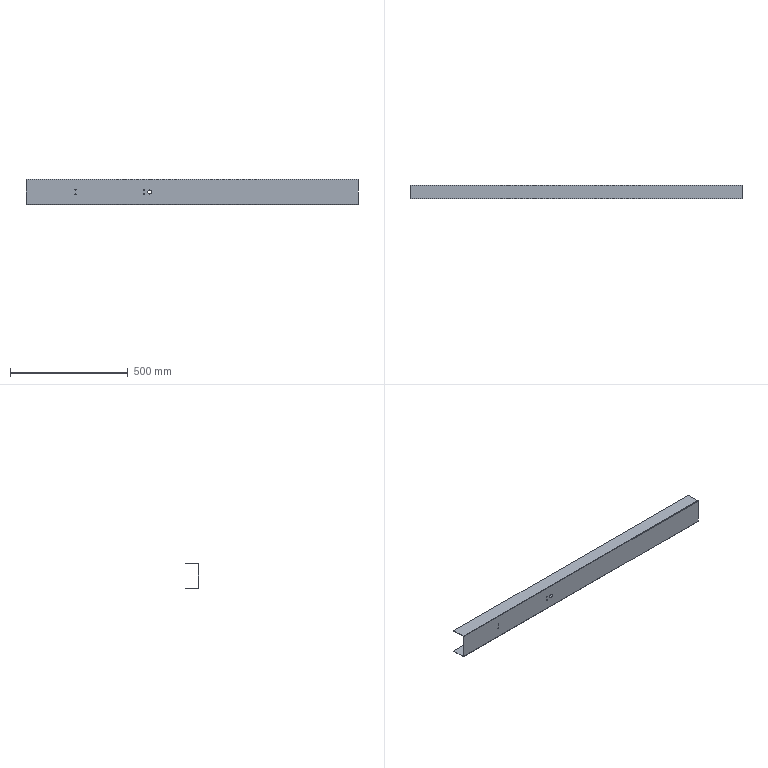Part | STEP file | Trunking Light 5 | 1 solid | 24 faces | box 1408 x 58 x 107 mm | volume 462641 mm3 | cylinder 14 | plane 10 | commonest cylinder face diameters 5 x8 0.2 x2 3.2 x2 17 x2
STEP:
#1=CARTESIAN_POINT('',(525.,-37.727,-23.631));
#2=VERTEX_POINT('',#1);
#3=CARTESIAN_POINT('',(525.,-37.727,-40.631));
#4=VERTEX_POINT('',#3);
#5=CARTESIAN_POINT('',(525.,-37.727,-32.131));
#6=DIRECTION('',(0.,-1.,0.));
#7=DIRECTION('',(0.,0.,-1.));
#8=AXIS2_PLACEMENT_3D('',#5,#6,#7);
#9=CIRCLE('',#8,8.5);
#10=EDGE_CURVE('',#2,#4,#9,.T.);
#11=ORIENTED_EDGE('',*,*,#10,.F.);
#12=CARTESIAN_POINT('',(525.,-39.227,-23.631));
#13=VERTEX_POINT('',#12);
#14=CARTESIAN_POINT('',(525.,-29.227,-23.631));
#15=DIRECTION('',(0.,-1.,0.));
#16=VECTOR('',#15,1000.);
#17=LINE('',#14,#16);
#18=EDGE_CURVE('',#2,#13,#17,.T.);
#19=ORIENTED_EDGE('',*,*,#18,.T.);
#20=CARTESIAN_POINT('',(525.,-39.227,-40.631));
#21=VERTEX_POINT('',#20);
#22=CARTESIAN_POINT('',(525.,-39.227,-32.131));
#23=DIRECTION('',(0.,-1.,0.));
#24=DIRECTION('',(0.,0.,-1.));
#25=AXIS2_PLACEMENT_3D('',#22,#23,#24);
#26=CIRCLE('',#25,8.5);
#27=EDGE_CURVE('',#13,#21,#26,.T.);
#28=ORIENTED_EDGE('',*,*,#27,.T.);
#29=CARTESIAN_POINT('',(525.,-29.227,-40.631));
#30=DIRECTION('',(0.,-1.,0.));
#31=VECTOR('',#30,1000.);
#32=LINE('',#29,#31);
#33=EDGE_CURVE('',#4,#21,#32,.T.);
#34=ORIENTED_EDGE('',*,*,#33,.F.);
#35=EDGE_LOOP('',(#11,#19,#28,#34));
#36=FACE_OUTER_BOUND('',#35,.T.);
#37=CARTESIAN_POINT('',(525.,-29.227,-32.131));
#38=DIRECTION('',(0.,-1.,0.));
#39=DIRECTION('',(0.,0.,-1.));
#40=AXIS2_PLACEMENT_3D('',#37,#38,#39);
#41=CYLINDRICAL_SURFACE('',#40,8.5);
#42=ADVANCED_FACE('',(#36),#41,.F.);
#43=CARTESIAN_POINT('',(500.,-37.727,-19.631));
#44=VERTEX_POINT('',#43);
#45=CARTESIAN_POINT('',(500.,-37.727,-24.631));
#46=VERTEX_POINT('',#45);
#47=CARTESIAN_POINT('',(500.,-37.727,-22.131));
#48=DIRECTION('',(0.,-1.,0.));
#49=DIRECTION('',(0.,0.,-1.));
#50=AXIS2_PLACEMENT_3D('',#47,#48,#49);
#51=CIRCLE('',#50,2.5);
#52=EDGE_CURVE('',#44,#46,#51,.T.);
#53=ORIENTED_EDGE('',*,*,#52,.F.);
#54=CARTESIAN_POINT('',(500.,-39.227,-19.631));
#55=VERTEX_POINT('',#54);
#56=CARTESIAN_POINT('',(500.,-29.227,-19.631));
#57=DIRECTION('',(0.,-1.,0.));
#58=VECTOR('',#57,1000.);
#59=LINE('',#56,#58);
#60=EDGE_CURVE('',#44,#55,#59,.T.);
#61=ORIENTED_EDGE('',*,*,#60,.T.);
#62=CARTESIAN_POINT('',(500.,-39.227,-24.631));
#63=VERTEX_POINT('',#62);
#64=CARTESIAN_POINT('',(500.,-39.227,-22.131));
#65=DIRECTION('',(0.,-1.,0.));
#66=DIRECTION('',(0.,0.,-1.));
#67=AXIS2_PLACEMENT_3D('',#64,#65,#66);
#68=CIRCLE('',#67,2.5);
#69=EDGE_CURVE('',#55,#63,#68,.T.);
#70=ORIENTED_EDGE('',*,*,#69,.T.);
#71=CARTESIAN_POINT('',(500.,-29.227,-24.631));
#72=DIRECTION('',(0.,-1.,0.));
#73=VECTOR('',#72,1000.);
#74=LINE('',#71,#73);
#75=EDGE_CURVE('',#46,#63,#74,.T.);
#76=ORIENTED_EDGE('',*,*,#75,.F.);
#77=EDGE_LOOP('',(#53,#61,#70,#76));
#78=FACE_OUTER_BOUND('',#77,.T.);
#79=CARTESIAN_POINT('',(500.,-29.227,-22.131));
#80=DIRECTION('',(0.,-1.,0.));
#81=DIRECTION('',(0.,0.,-1.));
#82=AXIS2_PLACEMENT_3D('',#79,#80,#81);
#83=CYLINDRICAL_SURFACE('',#82,2.5);
#84=ADVANCED_FACE('',(#78),#83,.F.);
#85=CARTESIAN_POINT('',(210.,-37.727,-19.631));
#86=VERTEX_POINT('',#85);
#87=CARTESIAN_POINT('',(210.,-37.727,-24.631));
#88=VERTEX_POINT('',#87);
#89=CARTESIAN_POINT('',(210.,-37.727,-22.131));
#90=DIRECTION('',(0.,-1.,0.));
#91=DIRECTION('',(0.,0.,-1.));
#92=AXIS2_PLACEMENT_3D('',#89,#90,#91);
#93=CIRCLE('',#92,2.5);
#94=EDGE_CURVE('',#86,#88,#93,.T.);
#95=ORIENTED_EDGE('',*,*,#94,.F.);
#96=CARTESIAN_POINT('',(210.,-39.227,-19.631));
#97=VERTEX_POINT('',#96);
#98=CARTESIAN_POINT('',(210.,-29.227,-19.631));
#99=DIRECTION('',(0.,-1.,0.));
#100=VECTOR('',#99,1000.);
#101=LINE('',#98,#100);
#102=EDGE_CURVE('',#86,#97,#101,.T.);
#103=ORIENTED_EDGE('',*,*,#102,.T.);
#104=CARTESIAN_POINT('',(210.,-39.227,-24.631));
#105=VERTEX_POINT('',#104);
#106=CARTESIAN_POINT('',(210.,-39.227,-22.131));
#107=DIRECTION('',(0.,-1.,0.));
#108=DIRECTION('',(0.,0.,-1.));
#109=AXIS2_PLACEMENT_3D('',#106,#107,#108);
#110=CIRCLE('',#109,2.5);
#111=EDGE_CURVE('',#97,#105,#110,.T.);
#112=ORIENTED_EDGE('',*,*,#111,.T.);
#113=CARTESIAN_POINT('',(210.,-29.227,-24.631));
#114=DIRECTION('',(0.,-1.,0.));
#115=VECTOR('',#114,1000.);
#116=LINE('',#113,#115);
#117=EDGE_CURVE('',#88,#105,#116,.T.);
#118=ORIENTED_EDGE('',*,*,#117,.F.);
#119=EDGE_LOOP('',(#95,#103,#112,#118));
#120=FACE_OUTER_BOUND('',#119,.T.);
#121=CARTESIAN_POINT('',(210.,-29.227,-22.131));
#122=DIRECTION('',(0.,-1.,0.));
#123=DIRECTION('',(0.,0.,-1.));
#124=AXIS2_PLACEMENT_3D('',#121,#122,#123);
#125=CYLINDRICAL_SURFACE('',#124,2.5);
#126=ADVANCED_FACE('',(#120),#125,.F.);
#127=CARTESIAN_POINT('',(210.,-37.727,-39.631));
#128=VERTEX_POINT('',#127);
#129=CARTESIAN_POINT('',(210.,-37.727,-44.631));
#130=VERTEX_POINT('',#129);
#131=CARTESIAN_POINT('',(210.,-37.727,-42.131));
#132=DIRECTION('',(0.,-1.,0.));
#133=DIRECTION('',(0.,0.,-1.));
#134=AXIS2_PLACEMENT_3D('',#131,#132,#133);
#135=CIRCLE('',#134,2.5);
#136=EDGE_CURVE('',#128,#130,#135,.T.);
#137=ORIENTED_EDGE('',*,*,#136,.F.);
#138=CARTESIAN_POINT('',(210.,-39.227,-39.631));
#139=VERTEX_POINT('',#138);
#140=CARTESIAN_POINT('',(210.,-29.227,-39.631));
#141=DIRECTION('',(0.,-1.,0.));
#142=VECTOR('',#141,1000.);
#143=LINE('',#140,#142);
#144=EDGE_CURVE('',#128,#139,#143,.T.);
#145=ORIENTED_EDGE('',*,*,#144,.T.);
#146=CARTESIAN_POINT('',(210.,-39.227,-44.631));
#147=VERTEX_POINT('',#146);
#148=CARTESIAN_POINT('',(210.,-39.227,-42.131));
#149=DIRECTION('',(0.,-1.,0.));
#150=DIRECTION('',(0.,0.,-1.));
#151=AXIS2_PLACEMENT_3D('',#148,#149,#150);
#152=CIRCLE('',#151,2.5);
#153=EDGE_CURVE('',#139,#147,#152,.T.);
#154=ORIENTED_EDGE('',*,*,#153,.T.);
#155=CARTESIAN_POINT('',(210.,-29.227,-44.631));
#156=DIRECTION('',(0.,-1.,0.));
#157=VECTOR('',#156,1000.);
#158=LINE('',#155,#157);
#159=EDGE_CURVE('',#130,#147,#158,.T.);
#160=ORIENTED_EDGE('',*,*,#159,.F.);
#161=EDGE_LOOP('',(#137,#145,#154,#160));
#162=FACE_OUTER_BOUND('',#161,.T.);
#163=CARTESIAN_POINT('',(210.,-29.227,-42.131));
#164=DIRECTION('',(0.,-1.,0.));
#165=DIRECTION('',(0.,0.,-1.));
#166=AXIS2_PLACEMENT_3D('',#163,#164,#165);
#167=CYLINDRICAL_SURFACE('',#166,2.5);
#168=ADVANCED_FACE('',(#162),#167,.F.);
#169=CARTESIAN_POINT('',(500.,-37.727,-39.631));
#170=VERTEX_POINT('',#169);
#171=CARTESIAN_POINT('',(500.,-37.727,-44.631));
#172=VERTEX_POINT('',#171);
#173=CARTESIAN_POINT('',(500.,-37.727,-42.131));
#174=DIRECTION('',(0.,-1.,0.));
#175=DIRECTION('',(0.,0.,-1.));
#176=AXIS2_PLACEMENT_3D('',#173,#174,#175);
#177=CIRCLE('',#176,2.5);
#178=EDGE_CURVE('',#170,#172,#177,.T.);
#179=ORIENTED_EDGE('',*,*,#178,.F.);
#180=CARTESIAN_POINT('',(500.,-39.227,-39.631));
#181=VERTEX_POINT('',#180);
#182=CARTESIAN_POINT('',(500.,-29.227,-39.631));
#183=DIRECTION('',(0.,-1.,0.));
#184=VECTOR('',#183,1000.);
#185=LINE('',#182,#184);
#186=EDGE_CURVE('',#170,#181,#185,.T.);
#187=ORIENTED_EDGE('',*,*,#186,.T.);
#188=CARTESIAN_POINT('',(500.,-39.227,-44.631));
#189=VERTEX_POINT('',#188);
#190=CARTESIAN_POINT('',(500.,-39.227,-42.131));
#191=DIRECTION('',(0.,-1.,0.));
#192=DIRECTION('',(0.,0.,-1.));
#193=AXIS2_PLACEMENT_3D('',#190,#191,#192);
#194=CIRCLE('',#193,2.5);
#195=EDGE_CURVE('',#181,#189,#194,.T.);
#196=ORIENTED_EDGE('',*,*,#195,.T.);
#197=CARTESIAN_POINT('',(500.,-29.227,-44.631));
#198=DIRECTION('',(0.,-1.,0.));
#199=VECTOR('',#198,1000.);
#200=LINE('',#197,#199);
#201=EDGE_CURVE('',#172,#189,#200,.T.);
#202=ORIENTED_EDGE('',*,*,#201,.F.);
#203=EDGE_LOOP('',(#179,#187,#196,#202));
#204=FACE_OUTER_BOUND('',#203,.T.);
#205=CARTESIAN_POINT('',(500.,-29.227,-42.131));
#206=DIRECTION('',(0.,-1.,0.));
#207=DIRECTION('',(0.,0.,-1.));
#208=AXIS2_PLACEMENT_3D('',#205,#206,#207);
#209=CYLINDRICAL_SURFACE('',#208,2.5);
#210=ADVANCED_FACE('',(#204),#209,.F.);
#211=CARTESIAN_POINT('',(1408.,-39.227,-84.031));
#212=VERTEX_POINT('',#211);
#213=CARTESIAN_POINT('',(0.,-39.227,-84.031));
#214=VERTEX_POINT('',#213);
#215=CARTESIAN_POINT('',(1408.,-39.227,-84.031));
#216=DIRECTION('',(-1.,0.,0.));
#217=VECTOR('',#216,1000.);
#218=LINE('',#215,#217);
#219=EDGE_CURVE('',#212,#214,#218,.T.);
#220=ORIENTED_EDGE('',*,*,#219,.F.);
#221=CARTESIAN_POINT('',(1408.,-39.227,19.769));
#222=VERTEX_POINT('',#221);
#223=CARTESIAN_POINT('',(1408.,-39.227,21.369));
#224=DIRECTION('',(0.,0.,-1.));
#225=VECTOR('',#224,1000.);
#226=LINE('',#223,#225);
#227=EDGE_CURVE('',#222,#212,#226,.T.);
#228=ORIENTED_EDGE('',*,*,#227,.F.);
#229=CARTESIAN_POINT('',(0.,-39.227,19.769));
#230=VERTEX_POINT('',#229);
#231=CARTESIAN_POINT('',(1408.,-39.227,19.769));
#232=DIRECTION('',(1.,0.,0.));
#233=VECTOR('',#232,1000.);
#234=LINE('',#231,#233);
#235=EDGE_CURVE('',#230,#222,#234,.T.);
#236=ORIENTED_EDGE('',*,*,#235,.F.);
#237=CARTESIAN_POINT('',(0.,-39.227,21.369));
#238=DIRECTION('',(0.,0.,1.));
#239=VECTOR('',#238,1000.);
#240=LINE('',#237,#239);
#241=EDGE_CURVE('',#214,#230,#240,.T.);
#242=ORIENTED_EDGE('',*,*,#241,.F.);
#243=EDGE_LOOP('',(#220,#228,#236,#242));
#244=FACE_OUTER_BOUND('',#243,.T.);
#245=CARTESIAN_POINT('',(525.,-39.227,-32.131));
#246=DIRECTION('',(0.,-1.,0.));
#247=DIRECTION('',(0.,0.,-1.));
#248=AXIS2_PLACEMENT_3D('',#245,#246,#247);
#249=CIRCLE('',#248,8.5);
#250=EDGE_CURVE('',#21,#13,#249,.T.);
#251=ORIENTED_EDGE('',*,*,#250,.F.);
#252=ORIENTED_EDGE('',*,*,#27,.F.);
#253=EDGE_LOOP('',(#251,#252));
#254=FACE_BOUND('',#253,.T.);
#255=CARTESIAN_POINT('',(500.,-39.227,-22.131));
#256=DIRECTION('',(0.,-1.,0.));
#257=DIRECTION('',(0.,0.,-1.));
#258=AXIS2_PLACEMENT_3D('',#255,#256,#257);
#259=CIRCLE('',#258,2.5);
#260=EDGE_CURVE('',#63,#55,#259,.T.);
#261=ORIENTED_EDGE('',*,*,#260,.F.);
#262=ORIENTED_EDGE('',*,*,#69,.F.);
#263=EDGE_LOOP('',(#261,#262));
#264=FACE_BOUND('',#263,.T.);
#265=CARTESIAN_POINT('',(210.,-39.227,-22.131));
#266=DIRECTION('',(0.,-1.,0.));
#267=DIRECTION('',(0.,0.,-1.));
#268=AXIS2_PLACEMENT_3D('',#265,#266,#267);
#269=CIRCLE('',#268,2.5);
#270=EDGE_CURVE('',#105,#97,#269,.T.);
#271=ORIENTED_EDGE('',*,*,#270,.F.);
#272=ORIENTED_EDGE('',*,*,#111,.F.);
#273=EDGE_LOOP('',(#271,#272));
#274=FACE_BOUND('',#273,.T.);
#275=CARTESIAN_POINT('',(210.,-39.227,-42.131));
#276=DIRECTION('',(0.,-1.,0.));
#277=DIRECTION('',(0.,0.,-1.));
#278=AXIS2_PLACEMENT_3D('',#275,#276,#277);
#279=CIRCLE('',#278,2.5);
#280=EDGE_CURVE('',#147,#139,#279,.T.);
#281=ORIENTED_EDGE('',*,*,#280,.F.);
#282=ORIENTED_EDGE('',*,*,#153,.F.);
#283=EDGE_LOOP('',(#281,#282));
#284=FACE_BOUND('',#283,.T.);
#285=CARTESIAN_POINT('',(500.,-39.227,-42.131));
#286=DIRECTION('',(0.,-1.,0.));
#287=DIRECTION('',(0.,0.,-1.));
#288=AXIS2_PLACEMENT_3D('',#285,#286,#287);
#289=CIRCLE('',#288,2.5);
#290=EDGE_CURVE('',#189,#181,#289,.T.);
#291=ORIENTED_EDGE('',*,*,#290,.F.);
#292=ORIENTED_EDGE('',*,*,#195,.F.);
#293=EDGE_LOOP('',(#291,#292));
#294=FACE_BOUND('',#293,.T.);
#295=CARTESIAN_POINT('',(1408.,-39.227,21.369));
#296=DIRECTION('',(0.,1.,0.));
#297=DIRECTION('',(0.,0.,1.));
#298=AXIS2_PLACEMENT_3D('',#295,#296,#297);
#299=PLANE('',#298);
#300=ADVANCED_FACE('',(#244,#254,#264,#274,#284,#294),#299,.F.);
#301=CARTESIAN_POINT('',(0.,-37.727,19.769));
#302=VERTEX_POINT('',#301);
#303=CARTESIAN_POINT('',(0.,-37.727,-84.031));
#304=VERTEX_POINT('',#303);
#305=CARTESIAN_POINT('',(0.,-37.727,19.869));
#306=DIRECTION('',(0.,0.,-1.));
#307=VECTOR('',#306,1000.);
#308=LINE('',#305,#307);
#309=EDGE_CURVE('',#302,#304,#308,.T.);
#310=ORIENTED_EDGE('',*,*,#309,.T.);
#311=CARTESIAN_POINT('',(0.,-37.627,-84.131));
#312=VERTEX_POINT('',#311);
#313=CARTESIAN_POINT('',(0.,-37.627,-84.031));
#314=DIRECTION('',(1.,0.,0.));
#315=DIRECTION('',(0.,0.,1.));
#316=AXIS2_PLACEMENT_3D('',#313,#314,#315);
#317=CIRCLE('',#316,0.1);
#318=EDGE_CURVE('',#304,#312,#317,.T.);
#319=ORIENTED_EDGE('',*,*,#318,.T.);
#320=CARTESIAN_POINT('',(0.,18.773,-84.131));
#321=VERTEX_POINT('',#320);
#322=CARTESIAN_POINT('',(0.,-37.727,-84.131));
#323=DIRECTION('',(0.,1.,0.));
#324=VECTOR('',#323,1000.);
#325=LINE('',#322,#324);
#326=EDGE_CURVE('',#312,#321,#325,.T.);
#327=ORIENTED_EDGE('',*,*,#326,.T.);
#328=CARTESIAN_POINT('',(0.,18.773,-85.631));
#329=VERTEX_POINT('',#328);
#330=CARTESIAN_POINT('',(0.,18.773,-84.031));
#331=DIRECTION('',(0.,0.,-1.));
#332=VECTOR('',#331,1000.);
#333=LINE('',#330,#332);
#334=EDGE_CURVE('',#321,#329,#333,.T.);
#335=ORIENTED_EDGE('',*,*,#334,.T.);
#336=CARTESIAN_POINT('',(0.,-37.627,-85.631));
#337=VERTEX_POINT('',#336);
#338=CARTESIAN_POINT('',(0.,-39.227,-85.631));
#339=DIRECTION('',(0.,-1.,0.));
#340=VECTOR('',#339,1000.);
#341=LINE('',#338,#340);
#342=EDGE_CURVE('',#329,#337,#341,.T.);
#343=ORIENTED_EDGE('',*,*,#342,.T.);
#344=CARTESIAN_POINT('',(0.,-37.627,-84.031));
#345=DIRECTION('',(1.,0.,0.));
#346=DIRECTION('',(0.,0.,1.));
#347=AXIS2_PLACEMENT_3D('',#344,#345,#346);
#348=CIRCLE('',#347,1.6);
#349=EDGE_CURVE('',#214,#337,#348,.T.);
#350=ORIENTED_EDGE('',*,*,#349,.F.);
#351=ORIENTED_EDGE('',*,*,#241,.T.);
#352=CARTESIAN_POINT('',(0.,-37.627,21.369));
#353=VERTEX_POINT('',#352);
#354=CARTESIAN_POINT('',(0.,-37.627,19.769));
#355=DIRECTION('',(1.,0.,0.));
#356=DIRECTION('',(0.,0.,1.));
#357=AXIS2_PLACEMENT_3D('',#354,#355,#356);
#358=CIRCLE('',#357,1.6);
#359=EDGE_CURVE('',#353,#230,#358,.T.);
#360=ORIENTED_EDGE('',*,*,#359,.F.);
#361=CARTESIAN_POINT('',(0.,18.773,21.369));
#362=VERTEX_POINT('',#361);
#363=CARTESIAN_POINT('',(0.,18.773,21.369));
#364=DIRECTION('',(0.,1.,0.));
#365=VECTOR('',#364,1000.);
#366=LINE('',#363,#365);
#367=EDGE_CURVE('',#353,#362,#366,.T.);
#368=ORIENTED_EDGE('',*,*,#367,.T.);
#369=CARTESIAN_POINT('',(0.,18.773,19.869));
#370=VERTEX_POINT('',#369);
#371=CARTESIAN_POINT('',(0.,18.773,-84.031));
#372=DIRECTION('',(0.,0.,1.));
#373=VECTOR('',#372,1000.);
#374=LINE('',#371,#373);
#375=EDGE_CURVE('',#370,#362,#374,.T.);
#376=ORIENTED_EDGE('',*,*,#375,.F.);
#377=CARTESIAN_POINT('',(0.,-37.627,19.869));
#378=VERTEX_POINT('',#377);
#379=CARTESIAN_POINT('',(0.,-37.627,19.869));
#380=DIRECTION('',(0.,1.,0.));
#381=VECTOR('',#380,1000.);
#382=LINE('',#379,#381);
#383=EDGE_CURVE('',#378,#370,#382,.T.);
#384=ORIENTED_EDGE('',*,*,#383,.F.);
#385=CARTESIAN_POINT('',(0.,-37.627,19.769));
#386=DIRECTION('',(1.,0.,0.));
#387=DIRECTION('',(0.,0.,1.));
#388=AXIS2_PLACEMENT_3D('',#385,#386,#387);
#389=CIRCLE('',#388,0.1);
#390=EDGE_CURVE('',#378,#302,#389,.T.);
#391=ORIENTED_EDGE('',*,*,#390,.T.);
#392=EDGE_LOOP('',(#310,#319,#327,#335,#343,#350,#351,#360,#368,#376,#384,#391));
#393=FACE_OUTER_BOUND('',#392,.T.);
#394=CARTESIAN_POINT('',(0.,-37.627,19.869));
#395=DIRECTION('',(-1.,0.,0.));
#396=DIRECTION('',(0.,0.,1.));
#397=AXIS2_PLACEMENT_3D('',#394,#395,#396);
#398=PLANE('',#397);
#399=ADVANCED_FACE('',(#393),#398,.T.);
#400=CARTESIAN_POINT('',(1408.,-37.627,-85.631));
#401=VERTEX_POINT('',#400);
#402=CARTESIAN_POINT('',(1408.,-37.627,-84.031));
#403=DIRECTION('',(-1.,0.,0.));
#404=DIRECTION('',(0.,0.,1.));
#405=AXIS2_PLACEMENT_3D('',#402,#403,#404);
#406=CIRCLE('',#405,1.6);
#407=EDGE_CURVE('',#401,#212,#406,.T.);
#408=ORIENTED_EDGE('',*,*,#407,.T.);
#409=ORIENTED_EDGE('',*,*,#219,.T.);
#410=ORIENTED_EDGE('',*,*,#349,.T.);
#411=CARTESIAN_POINT('',(1408.,-37.627,-85.631));
#412=DIRECTION('',(1.,0.,0.));
#413=VECTOR('',#412,1000.);
#414=LINE('',#411,#413);
#415=EDGE_CURVE('',#337,#401,#414,.T.);
#416=ORIENTED_EDGE('',*,*,#415,.T.);
#417=EDGE_LOOP('',(#408,#409,#410,#416));
#418=FACE_OUTER_BOUND('',#417,.T.);
#419=CARTESIAN_POINT('',(1408.,-37.627,-84.031));
#420=DIRECTION('',(-1.,0.,0.));
#421=DIRECTION('',(0.,0.,1.));
#422=AXIS2_PLACEMENT_3D('',#419,#420,#421);
#423=CYLINDRICAL_SURFACE('',#422,1.6);
#424=ADVANCED_FACE('',(#418),#423,.T.);
#425=CARTESIAN_POINT('',(1408.,-37.727,-84.031));
#426=VERTEX_POINT('',#425);
#427=CARTESIAN_POINT('',(1408.,-37.727,19.769));
#428=VERTEX_POINT('',#427);
#429=CARTESIAN_POINT('',(1408.,-37.727,-84.131));
#430=DIRECTION('',(0.,0.,1.));
#431=VECTOR('',#430,1000.);
#432=LINE('',#429,#431);
#433=EDGE_CURVE('',#426,#428,#432,.T.);
#434=ORIENTED_EDGE('',*,*,#433,.T.);
#435=CARTESIAN_POINT('',(1408.,-37.627,19.869));
#436=VERTEX_POINT('',#435);
#437=CARTESIAN_POINT('',(1408.,-37.627,19.769));
#438=DIRECTION('',(-1.,0.,0.));
#439=DIRECTION('',(0.,0.,1.));
#440=AXIS2_PLACEMENT_3D('',#437,#438,#439);
#441=CIRCLE('',#440,0.1);
#442=EDGE_CURVE('',#428,#436,#441,.T.);
#443=ORIENTED_EDGE('',*,*,#442,.T.);
#444=CARTESIAN_POINT('',(1408.,18.773,19.869));
#445=VERTEX_POINT('',#444);
#446=CARTESIAN_POINT('',(1408.,-37.727,19.869));
#447=DIRECTION('',(0.,1.,0.));
#448=VECTOR('',#447,1000.);
#449=LINE('',#446,#448);
#450=EDGE_CURVE('',#436,#445,#449,.T.);
#451=ORIENTED_EDGE('',*,*,#450,.T.);
#452=CARTESIAN_POINT('',(1408.,18.773,21.369));
#453=VERTEX_POINT('',#452);
#454=CARTESIAN_POINT('',(1408.,18.773,19.769));
#455=DIRECTION('',(0.,0.,1.));
#456=VECTOR('',#455,1000.);
#457=LINE('',#454,#456);
#458=EDGE_CURVE('',#445,#453,#457,.T.);
#459=ORIENTED_EDGE('',*,*,#458,.T.);
#460=CARTESIAN_POINT('',(1408.,-37.627,21.369));
#461=VERTEX_POINT('',#460);
#462=CARTESIAN_POINT('',(1408.,18.773,21.369));
#463=DIRECTION('',(0.,-1.,0.));
#464=VECTOR('',#463,1000.);
#465=LINE('',#462,#464);
#466=EDGE_CURVE('',#453,#461,#465,.T.);
#467=ORIENTED_EDGE('',*,*,#466,.T.);
#468=CARTESIAN_POINT('',(1408.,-37.627,19.769));
#469=DIRECTION('',(-1.,0.,0.));
#470=DIRECTION('',(0.,0.,1.));
#471=AXIS2_PLACEMENT_3D('',#468,#469,#470);
#472=CIRCLE('',#471,1.6);
#473=EDGE_CURVE('',#222,#461,#472,.T.);
#474=ORIENTED_EDGE('',*,*,#473,.F.);
#475=ORIENTED_EDGE('',*,*,#227,.T.);
#476=ORIENTED_EDGE('',*,*,#407,.F.);
#477=CARTESIAN_POINT('',(1408.,18.773,-85.631));
#478=VERTEX_POINT('',#477);
#479=CARTESIAN_POINT('',(1408.,-39.227,-85.631));
#480=DIRECTION('',(0.,1.,0.));
#481=VECTOR('',#480,1000.);
#482=LINE('',#479,#481);
#483=EDGE_CURVE('',#401,#478,#482,.T.);
#484=ORIENTED_EDGE('',*,*,#483,.T.);
#485=CARTESIAN_POINT('',(1408.,18.773,-84.131));
#486=VERTEX_POINT('',#485);
#487=CARTESIAN_POINT('',(1408.,18.773,-84.131));
#488=DIRECTION('',(0.,0.,-1.));
#489=VECTOR('',#488,1000.);
#490=LINE('',#487,#489);
#491=EDGE_CURVE('',#486,#478,#490,.T.);
#492=ORIENTED_EDGE('',*,*,#491,.F.);
#493=CARTESIAN_POINT('',(1408.,-37.627,-84.131));
#494=VERTEX_POINT('',#493);
#495=CARTESIAN_POINT('',(1408.,-37.627,-84.131));
#496=DIRECTION('',(0.,-1.,0.));
#497=VECTOR('',#496,1000.);
#498=LINE('',#495,#497);
#499=EDGE_CURVE('',#486,#494,#498,.T.);
#500=ORIENTED_EDGE('',*,*,#499,.T.);
#501=CARTESIAN_POINT('',(1408.,-37.627,-84.031));
#502=DIRECTION('',(-1.,0.,0.));
#503=DIRECTION('',(0.,0.,1.));
#504=AXIS2_PLACEMENT_3D('',#501,#502,#503);
#505=CIRCLE('',#504,0.1);
#506=EDGE_CURVE('',#494,#426,#505,.T.);
#507=ORIENTED_EDGE('',*,*,#506,.T.);
#508=EDGE_LOOP('',(#434,#443,#451,#459,#467,#474,#475,#476,#484,#492,#500,#507));
#509=FACE_OUTER_BOUND('',#508,.T.);
#510=CARTESIAN_POINT('',(1408.,-37.627,-84.131));
#511=DIRECTION('',(1.,0.,0.));
#512=DIRECTION('',(0.,0.,-1.));
#513=AXIS2_PLACEMENT_3D('',#510,#511,#512);
#514=PLANE('',#513);
#515=ADVANCED_FACE('',(#509),#514,.T.);
#516=ORIENTED_EDGE('',*,*,#473,.T.);
#517=CARTESIAN_POINT('',(1408.,-37.627,21.369));
#518=DIRECTION('',(-1.,0.,0.));
#519=VECTOR('',#518,1000.);
#520=LINE('',#517,#519);
#521=EDGE_CURVE('',#461,#353,#520,.T.);
#522=ORIENTED_EDGE('',*,*,#521,.T.);
#523=ORIENTED_EDGE('',*,*,#359,.T.);
#524=ORIENTED_EDGE('',*,*,#235,.T.);
#525=EDGE_LOOP('',(#516,#522,#523,#524));
#526=FACE_OUTER_BOUND('',#525,.T.);
#527=CARTESIAN_POINT('',(1408.,-37.627,19.769));
#528=DIRECTION('',(-1.,0.,0.));
#529=DIRECTION('',(0.,0.,1.));
#530=AXIS2_PLACEMENT_3D('',#527,#528,#529);
#531=CYLINDRICAL_SURFACE('',#530,1.6);
#532=ADVANCED_FACE('',(#526),#531,.T.);
#533=ORIENTED_EDGE('',*,*,#18,.F.);
#534=CARTESIAN_POINT('',(525.,-37.727,-32.131));
#535=DIRECTION('',(0.,-1.,0.));
#536=DIRECTION('',(0.,0.,-1.));
#537=AXIS2_PLACEMENT_3D('',#534,#535,#536);
#538=CIRCLE('',#537,8.5);
#539=EDGE_CURVE('',#4,#2,#538,.T.);
#540=ORIENTED_EDGE('',*,*,#539,.F.);
#541=ORIENTED_EDGE('',*,*,#33,.T.);
#542=ORIENTED_EDGE('',*,*,#250,.T.);
#543=EDGE_LOOP('',(#533,#540,#541,#542));
#544=FACE_OUTER_BOUND('',#543,.T.);
#545=CARTESIAN_POINT('',(525.,-29.227,-32.131));
#546=DIRECTION('',(0.,-1.,0.));
#547=DIRECTION('',(0.,0.,-1.));
#548=AXIS2_PLACEMENT_3D('',#545,#546,#547);
#549=CYLINDRICAL_SURFACE('',#548,8.5);
#550=ADVANCED_FACE('',(#544),#549,.F.);
#551=ORIENTED_EDGE('',*,*,#60,.F.);
#552=CARTESIAN_POINT('',(500.,-37.727,-22.131));
#553=DIRECTION('',(0.,-1.,0.));
#554=DIRECTION('',(0.,0.,-1.));
#555=AXIS2_PLACEMENT_3D('',#552,#553,#554);
#556=CIRCLE('',#555,2.5);
#557=EDGE_CURVE('',#46,#44,#556,.T.);
#558=ORIENTED_EDGE('',*,*,#557,.F.);
#559=ORIENTED_EDGE('',*,*,#75,.T.);
#560=ORIENTED_EDGE('',*,*,#260,.T.);
#561=EDGE_LOOP('',(#551,#558,#559,#560));
#562=FACE_OUTER_BOUND('',#561,.T.);
#563=CARTESIAN_POINT('',(500.,-29.227,-22.131));
#564=DIRECTION('',(0.,-1.,0.));
#565=DIRECTION('',(0.,0.,-1.));
#566=AXIS2_PLACEMENT_3D('',#563,#564,#565);
#567=CYLINDRICAL_SURFACE('',#566,2.5);
#568=ADVANCED_FACE('',(#562),#567,.F.);
#569=ORIENTED_EDGE('',*,*,#102,.F.);
#570=CARTESIAN_POINT('',(210.,-37.727,-22.131));
#571=DIRECTION('',(0.,-1.,0.));
#572=DIRECTION('',(0.,0.,-1.));
#573=AXIS2_PLACEMENT_3D('',#570,#571,#572);
#574=CIRCLE('',#573,2.5);
#575=EDGE_CURVE('',#88,#86,#574,.T.);
#576=ORIENTED_EDGE('',*,*,#575,.F.);
#577=ORIENTED_EDGE('',*,*,#117,.T.);
#578=ORIENTED_EDGE('',*,*,#270,.T.);
#579=EDGE_LOOP('',(#569,#576,#577,#578));
#580=FACE_OUTER_BOUND('',#579,.T.);
#581=CARTESIAN_POINT('',(210.,-29.227,-22.131));
#582=DIRECTION('',(0.,-1.,0.));
#583=DIRECTION('',(0.,0.,-1.));
#584=AXIS2_PLACEMENT_3D('',#581,#582,#583);
#585=CYLINDRICAL_SURFACE('',#584,2.5);
#586=ADVANCED_FACE('',(#580),#585,.F.);
#587=ORIENTED_EDGE('',*,*,#144,.F.);
#588=CARTESIAN_POINT('',(210.,-37.727,-42.131));
#589=DIRECTION('',(0.,-1.,0.));
#590=DIRECTION('',(0.,0.,-1.));
#591=AXIS2_PLACEMENT_3D('',#588,#589,#590);
#592=CIRCLE('',#591,2.5);
#593=EDGE_CURVE('',#130,#128,#592,.T.);
#594=ORIENTED_EDGE('',*,*,#593,.F.);
#595=ORIENTED_EDGE('',*,*,#159,.T.);
#596=ORIENTED_EDGE('',*,*,#280,.T.);
#597=EDGE_LOOP('',(#587,#594,#595,#596));
#598=FACE_OUTER_BOUND('',#597,.T.);
#599=CARTESIAN_POINT('',(210.,-29.227,-42.131));
#600=DIRECTION('',(0.,-1.,0.));
#601=DIRECTION('',(0.,0.,-1.));
#602=AXIS2_PLACEMENT_3D('',#599,#600,#601);
#603=CYLINDRICAL_SURFACE('',#602,2.5);
#604=ADVANCED_FACE('',(#598),#603,.F.);
#605=ORIENTED_EDGE('',*,*,#186,.F.);
#606=CARTESIAN_POINT('',(500.,-37.727,-42.131));
#607=DIRECTION('',(0.,-1.,0.));
#608=DIRECTION('',(0.,0.,-1.));
#609=AXIS2_PLACEMENT_3D('',#606,#607,#608);
#610=CIRCLE('',#609,2.5);
#611=EDGE_CURVE('',#172,#170,#610,.T.);
#612=ORIENTED_EDGE('',*,*,#611,.F.);
#613=ORIENTED_EDGE('',*,*,#201,.T.);
#614=ORIENTED_EDGE('',*,*,#290,.T.);
#615=EDGE_LOOP('',(#605,#612,#613,#614));
#616=FACE_OUTER_BOUND('',#615,.T.);
#617=CARTESIAN_POINT('',(500.,-29.227,-42.131));
#618=DIRECTION('',(0.,-1.,0.));
#619=DIRECTION('',(0.,0.,-1.));
#620=AXIS2_PLACEMENT_3D('',#617,#618,#619);
#621=CYLINDRICAL_SURFACE('',#620,2.5);
#622=ADVANCED_FACE('',(#616),#621,.F.);
#623=ORIENTED_EDGE('',*,*,#433,.F.);
#624=CARTESIAN_POINT('',(1408.,-37.727,-84.031));
#625=DIRECTION('',(-1.,0.,0.));
#626=VECTOR('',#625,1000.);
#627=LINE('',#624,#626);
#628=EDGE_CURVE('',#426,#304,#627,.T.);
#629=ORIENTED_EDGE('',*,*,#628,.T.);
#630=ORIENTED_EDGE('',*,*,#309,.F.);
#631=CARTESIAN_POINT('',(1408.,-37.727,19.769));
#632=DIRECTION('',(1.,0.,0.));
#633=VECTOR('',#632,1000.);
#634=LINE('',#631,#633);
#635=EDGE_CURVE('',#302,#428,#634,.T.);
#636=ORIENTED_EDGE('',*,*,#635,.T.);
#637=EDGE_LOOP('',(#623,#629,#630,#636));
#638=FACE_OUTER_BOUND('',#637,.T.);
#639=ORIENTED_EDGE('',*,*,#539,.T.);
#640=ORIENTED_EDGE('',*,*,#10,.T.);
#641=EDGE_LOOP('',(#639,#640));
#642=FACE_BOUND('',#641,.T.);
#643=ORIENTED_EDGE('',*,*,#557,.T.);
#644=ORIENTED_EDGE('',*,*,#52,.T.);
#645=EDGE_LOOP('',(#643,#644));
#646=FACE_BOUND('',#645,.T.);
#647=ORIENTED_EDGE('',*,*,#575,.T.);
#648=ORIENTED_EDGE('',*,*,#94,.T.);
#649=EDGE_LOOP('',(#647,#648));
#650=FACE_BOUND('',#649,.T.);
#651=ORIENTED_EDGE('',*,*,#593,.T.);
#652=ORIENTED_EDGE('',*,*,#136,.T.);
#653=EDGE_LOOP('',(#651,#652));
#654=FACE_BOUND('',#653,.T.);
#655=ORIENTED_EDGE('',*,*,#611,.T.);
#656=ORIENTED_EDGE('',*,*,#178,.T.);
#657=EDGE_LOOP('',(#655,#656));
#658=FACE_BOUND('',#657,.T.);
#659=CARTESIAN_POINT('',(1408.,-37.727,21.369));
#660=DIRECTION('',(0.,1.,0.));
#661=DIRECTION('',(0.,0.,1.));
#662=AXIS2_PLACEMENT_3D('',#659,#660,#661);
#663=PLANE('',#662);
#664=ADVANCED_FACE('',(#638,#642,#646,#650,#654,#658),#663,.T.);
#665=CARTESIAN_POINT('',(1408.,18.773,-85.631));
#666=DIRECTION('',(-1.,0.,0.));
#667=VECTOR('',#666,1000.);
#668=LINE('',#665,#667);
#669=EDGE_CURVE('',#478,#329,#668,.T.);
#670=ORIENTED_EDGE('',*,*,#669,.F.);
#671=ORIENTED_EDGE('',*,*,#483,.F.);
#672=ORIENTED_EDGE('',*,*,#415,.F.);
#673=ORIENTED_EDGE('',*,*,#342,.F.);
#674=EDGE_LOOP('',(#670,#671,#672,#673));
#675=FACE_OUTER_BOUND('',#674,.T.);
#676=CARTESIAN_POINT('',(1408.,-39.227,-85.631));
#677=DIRECTION('',(0.,0.,1.));
#678=DIRECTION('',(0.,-1.,0.));
#679=AXIS2_PLACEMENT_3D('',#676,#677,#678);
#680=PLANE('',#679);
#681=ADVANCED_FACE('',(#675),#680,.F.);
#682=ORIENTED_EDGE('',*,*,#521,.F.);
#683=ORIENTED_EDGE('',*,*,#466,.F.);
#684=CARTESIAN_POINT('',(1408.,18.773,21.369));
#685=DIRECTION('',(1.,0.,0.));
#686=VECTOR('',#685,1000.);
#687=LINE('',#684,#686);
#688=EDGE_CURVE('',#362,#453,#687,.T.);
#689=ORIENTED_EDGE('',*,*,#688,.F.);
#690=ORIENTED_EDGE('',*,*,#367,.F.);
#691=EDGE_LOOP('',(#682,#683,#689,#690));
#692=FACE_OUTER_BOUND('',#691,.T.);
#693=CARTESIAN_POINT('',(1408.,18.773,21.369));
#694=DIRECTION('',(0.,0.,-1.));
#695=DIRECTION('',(0.,1.,0.));
#696=AXIS2_PLACEMENT_3D('',#693,#694,#695);
#697=PLANE('',#696);
#698=ADVANCED_FACE('',(#692),#697,.F.);
#699=ORIENTED_EDGE('',*,*,#628,.F.);
#700=ORIENTED_EDGE('',*,*,#506,.F.);
#701=CARTESIAN_POINT('',(1408.,-37.627,-84.131));
#702=DIRECTION('',(1.,0.,0.));
#703=VECTOR('',#702,1000.);
#704=LINE('',#701,#703);
#705=EDGE_CURVE('',#312,#494,#704,.T.);
#706=ORIENTED_EDGE('',*,*,#705,.F.);
#707=ORIENTED_EDGE('',*,*,#318,.F.);
#708=EDGE_LOOP('',(#699,#700,#706,#707));
#709=FACE_OUTER_BOUND('',#708,.T.);
#710=CARTESIAN_POINT('',(1408.,-37.627,-84.031));
#711=DIRECTION('',(-1.,0.,0.));
#712=DIRECTION('',(0.,0.,1.));
#713=AXIS2_PLACEMENT_3D('',#710,#711,#712);
#714=CYLINDRICAL_SURFACE('',#713,0.1);
#715=ADVANCED_FACE('',(#709),#714,.F.);
#716=CARTESIAN_POINT('',(1408.,-37.627,19.869));
#717=DIRECTION('',(-1.,0.,0.));
#718=VECTOR('',#717,1000.);
#719=LINE('',#716,#718);
#720=EDGE_CURVE('',#436,#378,#719,.T.);
#721=ORIENTED_EDGE('',*,*,#720,.F.);
#722=ORIENTED_EDGE('',*,*,#442,.F.);
#723=ORIENTED_EDGE('',*,*,#635,.F.);
#724=ORIENTED_EDGE('',*,*,#390,.F.);
#725=EDGE_LOOP('',(#721,#722,#723,#724));
#726=FACE_OUTER_BOUND('',#725,.T.);
#727=CARTESIAN_POINT('',(1408.,-37.627,19.769));
#728=DIRECTION('',(-1.,0.,0.));
#729=DIRECTION('',(0.,0.,1.));
#730=AXIS2_PLACEMENT_3D('',#727,#728,#729);
#731=CYLINDRICAL_SURFACE('',#730,0.1);
#732=ADVANCED_FACE('',(#726),#731,.F.);
#733=ORIENTED_EDGE('',*,*,#491,.T.);
#734=ORIENTED_EDGE('',*,*,#669,.T.);
#735=ORIENTED_EDGE('',*,*,#334,.F.);
#736=CARTESIAN_POINT('',(1408.,18.773,-84.131));
#737=DIRECTION('',(1.,0.,0.));
#738=VECTOR('',#737,1000.);
#739=LINE('',#736,#738);
#740=EDGE_CURVE('',#321,#486,#739,.T.);
#741=ORIENTED_EDGE('',*,*,#740,.T.);
#742=EDGE_LOOP('',(#733,#734,#735,#741));
#743=FACE_OUTER_BOUND('',#742,.T.);
#744=CARTESIAN_POINT('',(1408.,18.773,-84.131));
#745=DIRECTION('',(0.,1.,0.));
#746=DIRECTION('',(0.,0.,1.));
#747=AXIS2_PLACEMENT_3D('',#744,#745,#746);
#748=PLANE('',#747);
#749=ADVANCED_FACE('',(#743),#748,.T.);
#750=ORIENTED_EDGE('',*,*,#458,.F.);
#751=CARTESIAN_POINT('',(1408.,18.773,19.869));
#752=DIRECTION('',(-1.,0.,0.));
#753=VECTOR('',#752,1000.);
#754=LINE('',#751,#753);
#755=EDGE_CURVE('',#445,#370,#754,.T.);
#756=ORIENTED_EDGE('',*,*,#755,.T.);
#757=ORIENTED_EDGE('',*,*,#375,.T.);
#758=ORIENTED_EDGE('',*,*,#688,.T.);
#759=EDGE_LOOP('',(#750,#756,#757,#758));
#760=FACE_OUTER_BOUND('',#759,.T.);
#761=CARTESIAN_POINT('',(1408.,18.773,21.369));
#762=DIRECTION('',(0.,1.,0.));
#763=DIRECTION('',(0.,0.,1.));
#764=AXIS2_PLACEMENT_3D('',#761,#762,#763);
#765=PLANE('',#764);
#766=ADVANCED_FACE('',(#760),#765,.T.);
#767=ORIENTED_EDGE('',*,*,#499,.F.);
#768=ORIENTED_EDGE('',*,*,#740,.F.);
#769=ORIENTED_EDGE('',*,*,#326,.F.);
#770=ORIENTED_EDGE('',*,*,#705,.T.);
#771=EDGE_LOOP('',(#767,#768,#769,#770));
#772=FACE_OUTER_BOUND('',#771,.T.);
#773=CARTESIAN_POINT('',(1408.,-39.227,-84.131));
#774=DIRECTION('',(0.,0.,1.));
#775=DIRECTION('',(0.,-1.,0.));
#776=AXIS2_PLACEMENT_3D('',#773,#774,#775);
#777=PLANE('',#776);
#778=ADVANCED_FACE('',(#772),#777,.T.);
#779=ORIENTED_EDGE('',*,*,#450,.F.);
#780=ORIENTED_EDGE('',*,*,#720,.T.);
#781=ORIENTED_EDGE('',*,*,#383,.T.);
#782=ORIENTED_EDGE('',*,*,#755,.F.);
#783=EDGE_LOOP('',(#779,#780,#781,#782));
#784=FACE_OUTER_BOUND('',#783,.T.);
#785=CARTESIAN_POINT('',(1408.,18.773,19.869));
#786=DIRECTION('',(0.,0.,-1.));
#787=DIRECTION('',(0.,1.,0.));
#788=AXIS2_PLACEMENT_3D('',#785,#786,#787);
#789=PLANE('',#788);
#790=ADVANCED_FACE('',(#784),#789,.T.);
#791=CLOSED_SHELL('',(#42,#84,#126,#168,#210,#300,#399,#424,#515,#532,#550,#568,#586,#604,#622,#664,#681,#698,#715,#732,#749,#766,#778,#790));
#792=MANIFOLD_SOLID_BREP('',#791);
#793=CARTESIAN_POINT('',(0.,0.,0.));
#794=DIRECTION('',(0.,0.,1.));
#795=DIRECTION('',(1.,0.,0.));
#796=AXIS2_PLACEMENT_3D('',#793,#794,#795);
#797=(LENGTH_UNIT()NAMED_UNIT(*)SI_UNIT(.MILLI.,.METRE.));
#798=UNCERTAINTY_MEASURE_WITH_UNIT(LENGTH_MEASURE(0.00001),#797,'','');
#799=(NAMED_UNIT(*)PLANE_ANGLE_UNIT()SI_UNIT($,.RADIAN.));
#800=(NAMED_UNIT(*)SI_UNIT($,.STERADIAN.)SOLID_ANGLE_UNIT());
#801=(GEOMETRIC_REPRESENTATION_CONTEXT(3)GLOBAL_UNCERTAINTY_ASSIGNED_CONTEXT((#798))GLOBAL_UNIT_ASSIGNED_CONTEXT((#797,#799,#800))REPRESENTATION_CONTEXT('',''));
#802=ADVANCED_BREP_SHAPE_REPRESENTATION('',(#792,#796),#801);